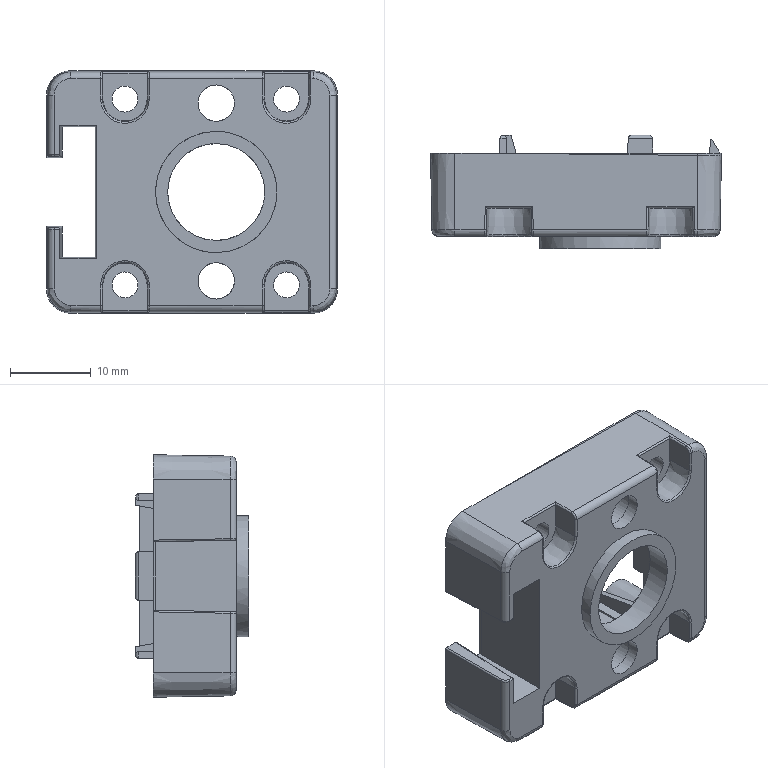Part | NX | 1 solid | 230 faces | box 36.005 x 14 x 30.01 mm | volume 3978 mm3 | plane 120 | cylinder 66 | cone 26 | spline 18 | commonest cylinder face diameters 0.4 x26 0.8 x15 1.6 x9 3.2 x4 3.14 x2 4.5 x2